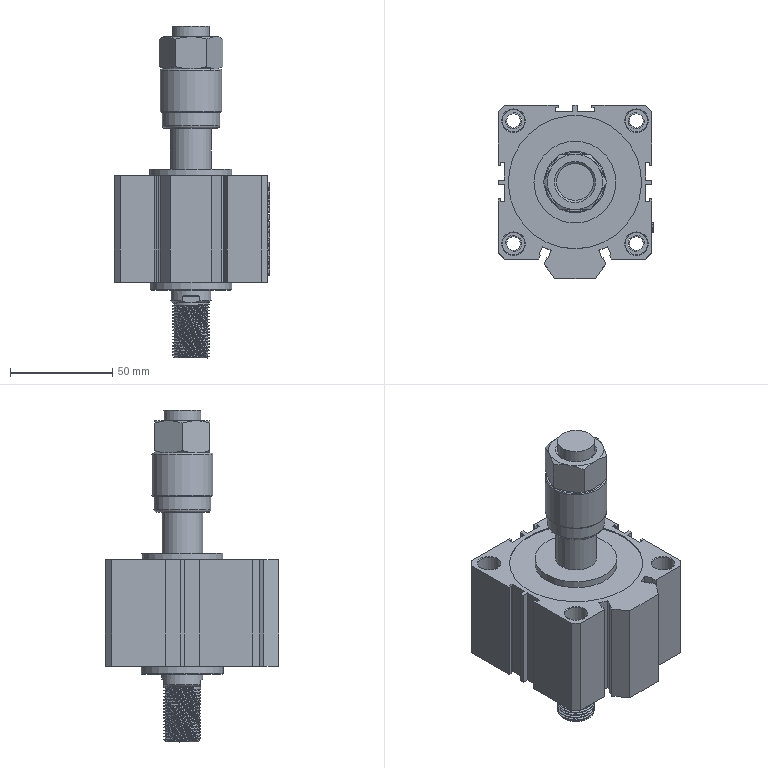Part | STEP file | YBQDJ-PD-15 | 1 solid | 367 faces | box 76 x 84.5 x 162 mm | volume 333527 mm3 | plane 171 | other 121 | cylinder 41 | cone 27 | torus 4 | spline 3 | commonest cylinder face diameters 11 x8 2.5 x4 6.75 x4 7.95 x4 8.05 x4 18 x3